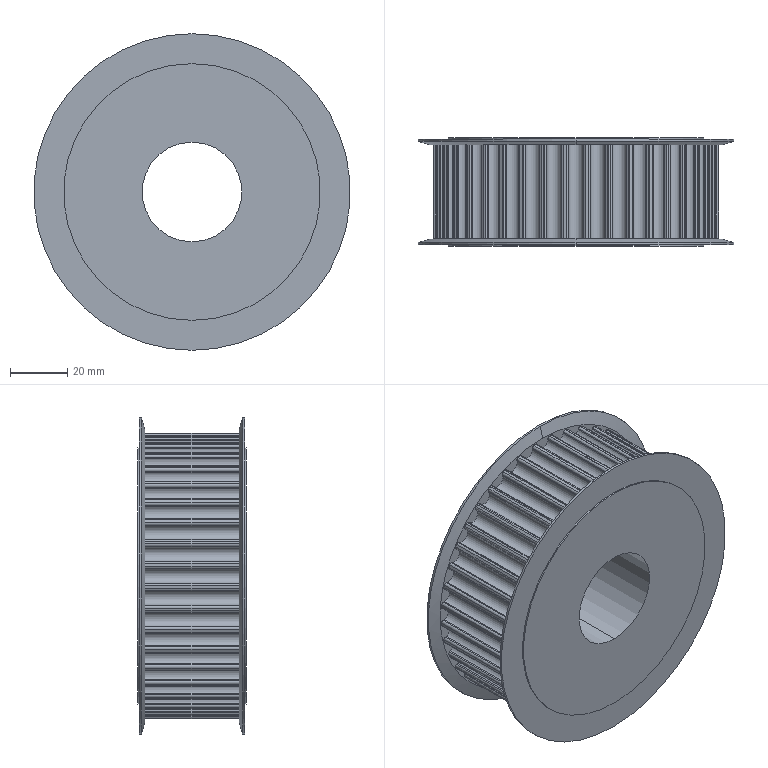Part | SolidWorks | features BaseBody 1 | 1 solid | 299 faces | box 111 x 38 x 111 mm | volume 247704 mm3 | cylinder 209 | plane 86 | cone 4 | commonest cylinder face diameters 1.62 x100 5.14 x59 100.49 x40 90 x4 111 x4 35 x2